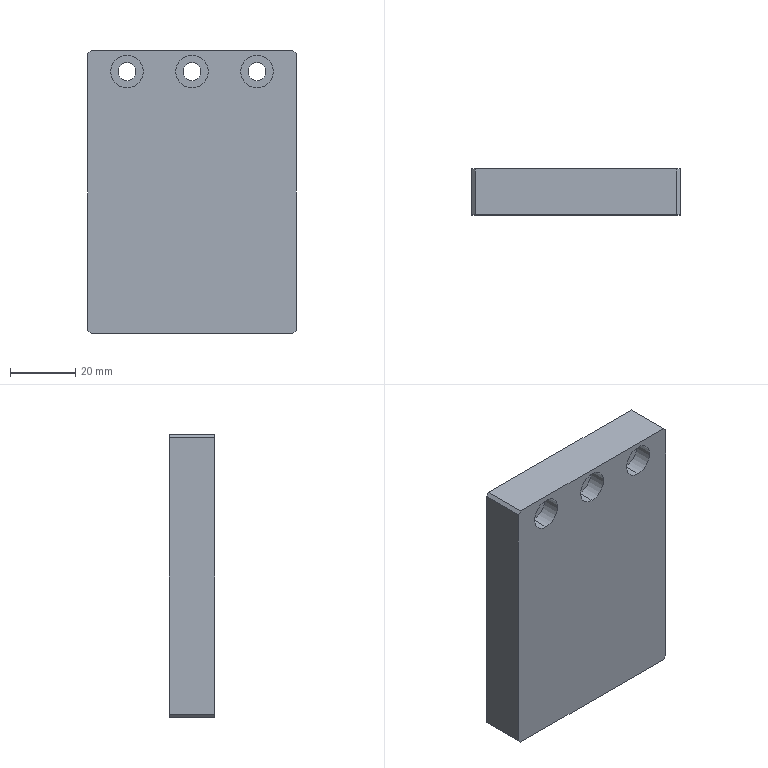Part | SolidWorks | features HoleWzd 2, Chamfer 1, Extrusion 1 | 1 solid | 37 faces | box 64 x 14 x 87 mm | volume 75198 mm3 | cylinder 18 | plane 13 | cone 6 | commonest cylinder face diameters 5 x6 5.5 x6 10 x6
STEP:
#1=CARTESIAN_POINT('',(32.5,-67.68,13.5));
#2=VERTEX_POINT('',#1);
#3=CARTESIAN_POINT('',(27.5,-67.68,13.5));
#4=VERTEX_POINT('',#3);
#5=CARTESIAN_POINT('',(30.,-67.68,13.5));
#6=DIRECTION('',(0.,0.,-1.));
#7=DIRECTION('',(-1.,0.,0.));
#8=AXIS2_PLACEMENT_3D('',#5,#6,#7);
#9=CIRCLE('',#8,2.5);
#10=EDGE_CURVE('',#2,#4,#9,.T.);
#11=ORIENTED_EDGE('',*,*,#10,.F.);
#12=CARTESIAN_POINT('',(32.5,-67.68,0.));
#13=VERTEX_POINT('',#12);
#14=CARTESIAN_POINT('',(32.5,-67.68,0.));
#15=DIRECTION('',(0.,0.,-1.));
#16=VECTOR('',#15,1000.);
#17=LINE('',#14,#16);
#18=EDGE_CURVE('',#2,#13,#17,.T.);
#19=ORIENTED_EDGE('',*,*,#18,.T.);
#20=CARTESIAN_POINT('',(27.5,-67.68,0.));
#21=VERTEX_POINT('',#20);
#22=CARTESIAN_POINT('',(30.,-67.68,0.));
#23=DIRECTION('',(0.,0.,-1.));
#24=DIRECTION('',(-1.,0.,0.));
#25=AXIS2_PLACEMENT_3D('',#22,#23,#24);
#26=CIRCLE('',#25,2.5);
#27=EDGE_CURVE('',#13,#21,#26,.T.);
#28=ORIENTED_EDGE('',*,*,#27,.T.);
#29=CARTESIAN_POINT('',(27.5,-67.68,0.));
#30=DIRECTION('',(0.,0.,-1.));
#31=VECTOR('',#30,1000.);
#32=LINE('',#29,#31);
#33=EDGE_CURVE('',#4,#21,#32,.T.);
#34=ORIENTED_EDGE('',*,*,#33,.F.);
#35=EDGE_LOOP('',(#11,#19,#28,#34));
#36=FACE_OUTER_BOUND('',#35,.T.);
#37=CARTESIAN_POINT('',(30.,-67.68,0.));
#38=DIRECTION('',(0.,0.,-1.));
#39=DIRECTION('',(-1.,0.,0.));
#40=AXIS2_PLACEMENT_3D('',#37,#38,#39);
#41=CYLINDRICAL_SURFACE('',#40,2.5);
#42=ADVANCED_FACE('',(#36),#41,.F.);
#43=CARTESIAN_POINT('',(30.,-67.68,15.002));
#44=VERTEX_POINT('',#43);
#45=CARTESIAN_POINT('',(27.5,-67.68,13.5));
#46=DIRECTION('',(-0.8572,0.,-0.515));
#47=VECTOR('',#46,1000.);
#48=LINE('',#45,#47);
#49=EDGE_CURVE('',#44,#4,#48,.T.);
#50=ORIENTED_EDGE('',*,*,#49,.F.);
#51=CARTESIAN_POINT('',(32.5,-67.68,13.5));
#52=DIRECTION('',(0.8572,0.,-0.515));
#53=VECTOR('',#52,1000.);
#54=LINE('',#51,#53);
#55=EDGE_CURVE('',#44,#2,#54,.T.);
#56=ORIENTED_EDGE('',*,*,#55,.T.);
#57=ORIENTED_EDGE('',*,*,#10,.T.);
#58=EDGE_LOOP('',(#50,#56,#57));
#59=FACE_OUTER_BOUND('',#58,.T.);
#60=CARTESIAN_POINT('',(30.,-67.68,13.5));
#61=DIRECTION('',(0.,0.,-1.));
#62=DIRECTION('',(-1.,0.,0.));
#63=AXIS2_PLACEMENT_3D('',#60,#61,#62);
#64=CONICAL_SURFACE('',#63,2.5,1.03);
#65=ADVANCED_FACE('',(#59),#64,.F.);
#66=CARTESIAN_POINT('',(12.5,-67.68,13.5));
#67=VERTEX_POINT('',#66);
#68=CARTESIAN_POINT('',(7.5,-67.68,13.5));
#69=VERTEX_POINT('',#68);
#70=CARTESIAN_POINT('',(10.,-67.68,13.5));
#71=DIRECTION('',(0.,0.,-1.));
#72=DIRECTION('',(-1.,0.,0.));
#73=AXIS2_PLACEMENT_3D('',#70,#71,#72);
#74=CIRCLE('',#73,2.5);
#75=EDGE_CURVE('',#67,#69,#74,.T.);
#76=ORIENTED_EDGE('',*,*,#75,.F.);
#77=CARTESIAN_POINT('',(12.5,-67.68,0.));
#78=VERTEX_POINT('',#77);
#79=CARTESIAN_POINT('',(12.5,-67.68,0.));
#80=DIRECTION('',(0.,0.,-1.));
#81=VECTOR('',#80,1000.);
#82=LINE('',#79,#81);
#83=EDGE_CURVE('',#67,#78,#82,.T.);
#84=ORIENTED_EDGE('',*,*,#83,.T.);
#85=CARTESIAN_POINT('',(7.5,-67.68,0.));
#86=VERTEX_POINT('',#85);
#87=CARTESIAN_POINT('',(10.,-67.68,0.));
#88=DIRECTION('',(0.,0.,-1.));
#89=DIRECTION('',(-1.,0.,0.));
#90=AXIS2_PLACEMENT_3D('',#87,#88,#89);
#91=CIRCLE('',#90,2.5);
#92=EDGE_CURVE('',#78,#86,#91,.T.);
#93=ORIENTED_EDGE('',*,*,#92,.T.);
#94=CARTESIAN_POINT('',(7.5,-67.68,0.));
#95=DIRECTION('',(0.,0.,-1.));
#96=VECTOR('',#95,1000.);
#97=LINE('',#94,#96);
#98=EDGE_CURVE('',#69,#86,#97,.T.);
#99=ORIENTED_EDGE('',*,*,#98,.F.);
#100=EDGE_LOOP('',(#76,#84,#93,#99));
#101=FACE_OUTER_BOUND('',#100,.T.);
#102=CARTESIAN_POINT('',(10.,-67.68,0.));
#103=DIRECTION('',(0.,0.,-1.));
#104=DIRECTION('',(-1.,0.,0.));
#105=AXIS2_PLACEMENT_3D('',#102,#103,#104);
#106=CYLINDRICAL_SURFACE('',#105,2.5);
#107=ADVANCED_FACE('',(#101),#106,.F.);
#108=CARTESIAN_POINT('',(10.,-67.68,15.002));
#109=VERTEX_POINT('',#108);
#110=CARTESIAN_POINT('',(7.5,-67.68,13.5));
#111=DIRECTION('',(-0.8572,0.,-0.515));
#112=VECTOR('',#111,1000.);
#113=LINE('',#110,#112);
#114=EDGE_CURVE('',#109,#69,#113,.T.);
#115=ORIENTED_EDGE('',*,*,#114,.F.);
#116=CARTESIAN_POINT('',(12.5,-67.68,13.5));
#117=DIRECTION('',(0.8572,0.,-0.515));
#118=VECTOR('',#117,1000.);
#119=LINE('',#116,#118);
#120=EDGE_CURVE('',#109,#67,#119,.T.);
#121=ORIENTED_EDGE('',*,*,#120,.T.);
#122=ORIENTED_EDGE('',*,*,#75,.T.);
#123=EDGE_LOOP('',(#115,#121,#122));
#124=FACE_OUTER_BOUND('',#123,.T.);
#125=CARTESIAN_POINT('',(10.,-67.68,13.5));
#126=DIRECTION('',(0.,0.,-1.));
#127=DIRECTION('',(-1.,0.,0.));
#128=AXIS2_PLACEMENT_3D('',#125,#126,#127);
#129=CONICAL_SURFACE('',#128,2.5,1.03);
#130=ADVANCED_FACE('',(#124),#129,.F.);
#131=CARTESIAN_POINT('',(-7.5,-67.68,13.5));
#132=VERTEX_POINT('',#131);
#133=CARTESIAN_POINT('',(-12.5,-67.68,13.5));
#134=VERTEX_POINT('',#133);
#135=CARTESIAN_POINT('',(-10.,-67.68,13.5));
#136=DIRECTION('',(0.,0.,-1.));
#137=DIRECTION('',(-1.,0.,0.));
#138=AXIS2_PLACEMENT_3D('',#135,#136,#137);
#139=CIRCLE('',#138,2.5);
#140=EDGE_CURVE('',#132,#134,#139,.T.);
#141=ORIENTED_EDGE('',*,*,#140,.F.);
#142=CARTESIAN_POINT('',(-7.5,-67.68,0.));
#143=VERTEX_POINT('',#142);
#144=CARTESIAN_POINT('',(-7.5,-67.68,0.));
#145=DIRECTION('',(0.,0.,-1.));
#146=VECTOR('',#145,1000.);
#147=LINE('',#144,#146);
#148=EDGE_CURVE('',#132,#143,#147,.T.);
#149=ORIENTED_EDGE('',*,*,#148,.T.);
#150=CARTESIAN_POINT('',(-12.5,-67.68,0.));
#151=VERTEX_POINT('',#150);
#152=CARTESIAN_POINT('',(-10.,-67.68,0.));
#153=DIRECTION('',(0.,0.,-1.));
#154=DIRECTION('',(-1.,0.,0.));
#155=AXIS2_PLACEMENT_3D('',#152,#153,#154);
#156=CIRCLE('',#155,2.5);
#157=EDGE_CURVE('',#143,#151,#156,.T.);
#158=ORIENTED_EDGE('',*,*,#157,.T.);
#159=CARTESIAN_POINT('',(-12.5,-67.68,0.));
#160=DIRECTION('',(0.,0.,-1.));
#161=VECTOR('',#160,1000.);
#162=LINE('',#159,#161);
#163=EDGE_CURVE('',#134,#151,#162,.T.);
#164=ORIENTED_EDGE('',*,*,#163,.F.);
#165=EDGE_LOOP('',(#141,#149,#158,#164));
#166=FACE_OUTER_BOUND('',#165,.T.);
#167=CARTESIAN_POINT('',(-10.,-67.68,0.));
#168=DIRECTION('',(0.,0.,-1.));
#169=DIRECTION('',(-1.,0.,0.));
#170=AXIS2_PLACEMENT_3D('',#167,#168,#169);
#171=CYLINDRICAL_SURFACE('',#170,2.5);
#172=ADVANCED_FACE('',(#166),#171,.F.);
#173=CARTESIAN_POINT('',(-10.,-67.68,15.002));
#174=VERTEX_POINT('',#173);
#175=CARTESIAN_POINT('',(-12.5,-67.68,13.5));
#176=DIRECTION('',(-0.8572,0.,-0.515));
#177=VECTOR('',#176,1000.);
#178=LINE('',#175,#177);
#179=EDGE_CURVE('',#174,#134,#178,.T.);
#180=ORIENTED_EDGE('',*,*,#179,.F.);
#181=CARTESIAN_POINT('',(-7.5,-67.68,13.5));
#182=DIRECTION('',(0.8572,0.,-0.515));
#183=VECTOR('',#182,1000.);
#184=LINE('',#181,#183);
#185=EDGE_CURVE('',#174,#132,#184,.T.);
#186=ORIENTED_EDGE('',*,*,#185,.T.);
#187=ORIENTED_EDGE('',*,*,#140,.T.);
#188=EDGE_LOOP('',(#180,#186,#187));
#189=FACE_OUTER_BOUND('',#188,.T.);
#190=CARTESIAN_POINT('',(-10.,-67.68,13.5));
#191=DIRECTION('',(0.,0.,-1.));
#192=DIRECTION('',(-1.,0.,0.));
#193=AXIS2_PLACEMENT_3D('',#190,#191,#192);
#194=CONICAL_SURFACE('',#193,2.5,1.03);
#195=ADVANCED_FACE('',(#189),#194,.F.);
#196=CARTESIAN_POINT('',(-10.,-69.18,85.5));
#197=VERTEX_POINT('',#196);
#198=CARTESIAN_POINT('',(-10.,-69.18,75.5));
#199=VERTEX_POINT('',#198);
#200=CARTESIAN_POINT('',(-10.,-69.18,80.5));
#201=DIRECTION('',(0.,-1.,0.));
#202=DIRECTION('',(0.,0.,-1.));
#203=AXIS2_PLACEMENT_3D('',#200,#201,#202);
#204=CIRCLE('',#203,5.);
#205=EDGE_CURVE('',#197,#199,#204,.T.);
#206=ORIENTED_EDGE('',*,*,#205,.F.);
#207=CARTESIAN_POINT('',(-10.,-74.68,85.5));
#208=VERTEX_POINT('',#207);
#209=CARTESIAN_POINT('',(-10.,-74.68,85.5));
#210=DIRECTION('',(0.,-1.,0.));
#211=VECTOR('',#210,1000.);
#212=LINE('',#209,#211);
#213=EDGE_CURVE('',#197,#208,#212,.T.);
#214=ORIENTED_EDGE('',*,*,#213,.T.);
#215=CARTESIAN_POINT('',(-10.,-74.68,75.5));
#216=VERTEX_POINT('',#215);
#217=CARTESIAN_POINT('',(-10.,-74.68,80.5));
#218=DIRECTION('',(0.,-1.,0.));
#219=DIRECTION('',(0.,0.,-1.));
#220=AXIS2_PLACEMENT_3D('',#217,#218,#219);
#221=CIRCLE('',#220,5.);
#222=EDGE_CURVE('',#208,#216,#221,.T.);
#223=ORIENTED_EDGE('',*,*,#222,.T.);
#224=CARTESIAN_POINT('',(-10.,-74.68,75.5));
#225=DIRECTION('',(0.,-1.,0.));
#226=VECTOR('',#225,1000.);
#227=LINE('',#224,#226);
#228=EDGE_CURVE('',#199,#216,#227,.T.);
#229=ORIENTED_EDGE('',*,*,#228,.F.);
#230=EDGE_LOOP('',(#206,#214,#223,#229));
#231=FACE_OUTER_BOUND('',#230,.T.);
#232=CARTESIAN_POINT('',(-10.,-74.68,80.5));
#233=DIRECTION('',(0.,-1.,0.));
#234=DIRECTION('',(0.,0.,-1.));
#235=AXIS2_PLACEMENT_3D('',#232,#233,#234);
#236=CYLINDRICAL_SURFACE('',#235,5.);
#237=ADVANCED_FACE('',(#231),#236,.F.);
#238=CARTESIAN_POINT('',(-10.,-60.68,83.25));
#239=VERTEX_POINT('',#238);
#240=CARTESIAN_POINT('',(-10.,-60.68,77.75));
#241=VERTEX_POINT('',#240);
#242=CARTESIAN_POINT('',(-10.,-60.68,80.5));
#243=DIRECTION('',(0.,-1.,0.));
#244=DIRECTION('',(0.,0.,-1.));
#245=AXIS2_PLACEMENT_3D('',#242,#243,#244);
#246=CIRCLE('',#245,2.75);
#247=EDGE_CURVE('',#239,#241,#246,.T.);
#248=ORIENTED_EDGE('',*,*,#247,.F.);
#249=CARTESIAN_POINT('',(-10.,-69.18,83.25));
#250=VERTEX_POINT('',#249);
#251=CARTESIAN_POINT('',(-10.,-74.68,83.25));
#252=DIRECTION('',(0.,-1.,0.));
#253=VECTOR('',#252,1000.);
#254=LINE('',#251,#253);
#255=EDGE_CURVE('',#239,#250,#254,.T.);
#256=ORIENTED_EDGE('',*,*,#255,.T.);
#257=CARTESIAN_POINT('',(-10.,-69.18,77.75));
#258=VERTEX_POINT('',#257);
#259=CARTESIAN_POINT('',(-10.,-69.18,80.5));
#260=DIRECTION('',(0.,-1.,0.));
#261=DIRECTION('',(0.,0.,-1.));
#262=AXIS2_PLACEMENT_3D('',#259,#260,#261);
#263=CIRCLE('',#262,2.75);
#264=EDGE_CURVE('',#250,#258,#263,.T.);
#265=ORIENTED_EDGE('',*,*,#264,.T.);
#266=CARTESIAN_POINT('',(-10.,-74.68,77.75));
#267=DIRECTION('',(0.,-1.,0.));
#268=VECTOR('',#267,1000.);
#269=LINE('',#266,#268);
#270=EDGE_CURVE('',#241,#258,#269,.T.);
#271=ORIENTED_EDGE('',*,*,#270,.F.);
#272=EDGE_LOOP('',(#248,#256,#265,#271));
#273=FACE_OUTER_BOUND('',#272,.T.);
#274=CARTESIAN_POINT('',(-10.,-74.68,80.5));
#275=DIRECTION('',(0.,-1.,0.));
#276=DIRECTION('',(0.,0.,-1.));
#277=AXIS2_PLACEMENT_3D('',#274,#275,#276);
#278=CYLINDRICAL_SURFACE('',#277,2.75);
#279=ADVANCED_FACE('',(#273),#278,.F.);
#280=CARTESIAN_POINT('',(10.,-69.18,85.5));
#281=VERTEX_POINT('',#280);
#282=CARTESIAN_POINT('',(10.,-69.18,75.5));
#283=VERTEX_POINT('',#282);
#284=CARTESIAN_POINT('',(10.,-69.18,80.5));
#285=DIRECTION('',(0.,-1.,0.));
#286=DIRECTION('',(0.,0.,-1.));
#287=AXIS2_PLACEMENT_3D('',#284,#285,#286);
#288=CIRCLE('',#287,5.);
#289=EDGE_CURVE('',#281,#283,#288,.T.);
#290=ORIENTED_EDGE('',*,*,#289,.F.);
#291=CARTESIAN_POINT('',(10.,-74.68,85.5));
#292=VERTEX_POINT('',#291);
#293=CARTESIAN_POINT('',(10.,-74.68,85.5));
#294=DIRECTION('',(0.,-1.,0.));
#295=VECTOR('',#294,1000.);
#296=LINE('',#293,#295);
#297=EDGE_CURVE('',#281,#292,#296,.T.);
#298=ORIENTED_EDGE('',*,*,#297,.T.);
#299=CARTESIAN_POINT('',(10.,-74.68,75.5));
#300=VERTEX_POINT('',#299);
#301=CARTESIAN_POINT('',(10.,-74.68,80.5));
#302=DIRECTION('',(0.,-1.,0.));
#303=DIRECTION('',(0.,0.,-1.));
#304=AXIS2_PLACEMENT_3D('',#301,#302,#303);
#305=CIRCLE('',#304,5.);
#306=EDGE_CURVE('',#292,#300,#305,.T.);
#307=ORIENTED_EDGE('',*,*,#306,.T.);
#308=CARTESIAN_POINT('',(10.,-74.68,75.5));
#309=DIRECTION('',(0.,-1.,0.));
#310=VECTOR('',#309,1000.);
#311=LINE('',#308,#310);
#312=EDGE_CURVE('',#283,#300,#311,.T.);
#313=ORIENTED_EDGE('',*,*,#312,.F.);
#314=EDGE_LOOP('',(#290,#298,#307,#313));
#315=FACE_OUTER_BOUND('',#314,.T.);
#316=CARTESIAN_POINT('',(10.,-74.68,80.5));
#317=DIRECTION('',(0.,-1.,0.));
#318=DIRECTION('',(0.,0.,-1.));
#319=AXIS2_PLACEMENT_3D('',#316,#317,#318);
#320=CYLINDRICAL_SURFACE('',#319,5.);
#321=ADVANCED_FACE('',(#315),#320,.F.);
#322=CARTESIAN_POINT('',(10.,-60.68,83.25));
#323=VERTEX_POINT('',#322);
#324=CARTESIAN_POINT('',(10.,-60.68,77.75));
#325=VERTEX_POINT('',#324);
#326=CARTESIAN_POINT('',(10.,-60.68,80.5));
#327=DIRECTION('',(0.,-1.,0.));
#328=DIRECTION('',(0.,0.,-1.));
#329=AXIS2_PLACEMENT_3D('',#326,#327,#328);
#330=CIRCLE('',#329,2.75);
#331=EDGE_CURVE('',#323,#325,#330,.T.);
#332=ORIENTED_EDGE('',*,*,#331,.F.);
#333=CARTESIAN_POINT('',(10.,-69.18,83.25));
#334=VERTEX_POINT('',#333);
#335=CARTESIAN_POINT('',(10.,-74.68,83.25));
#336=DIRECTION('',(0.,-1.,0.));
#337=VECTOR('',#336,1000.);
#338=LINE('',#335,#337);
#339=EDGE_CURVE('',#323,#334,#338,.T.);
#340=ORIENTED_EDGE('',*,*,#339,.T.);
#341=CARTESIAN_POINT('',(10.,-69.18,77.75));
#342=VERTEX_POINT('',#341);
#343=CARTESIAN_POINT('',(10.,-69.18,80.5));
#344=DIRECTION('',(0.,-1.,0.));
#345=DIRECTION('',(0.,0.,-1.));
#346=AXIS2_PLACEMENT_3D('',#343,#344,#345);
#347=CIRCLE('',#346,2.75);
#348=EDGE_CURVE('',#334,#342,#347,.T.);
#349=ORIENTED_EDGE('',*,*,#348,.T.);
#350=CARTESIAN_POINT('',(10.,-74.68,77.75));
#351=DIRECTION('',(0.,-1.,0.));
#352=VECTOR('',#351,1000.);
#353=LINE('',#350,#352);
#354=EDGE_CURVE('',#325,#342,#353,.T.);
#355=ORIENTED_EDGE('',*,*,#354,.F.);
#356=EDGE_LOOP('',(#332,#340,#349,#355));
#357=FACE_OUTER_BOUND('',#356,.T.);
#358=CARTESIAN_POINT('',(10.,-74.68,80.5));
#359=DIRECTION('',(0.,-1.,0.));
#360=DIRECTION('',(0.,0.,-1.));
#361=AXIS2_PLACEMENT_3D('',#358,#359,#360);
#362=CYLINDRICAL_SURFACE('',#361,2.75);
#363=ADVANCED_FACE('',(#357),#362,.F.);
#364=CARTESIAN_POINT('',(30.,-69.18,85.5));
#365=VERTEX_POINT('',#364);
#366=CARTESIAN_POINT('',(30.,-69.18,75.5));
#367=VERTEX_POINT('',#366);
#368=CARTESIAN_POINT('',(30.,-69.18,80.5));
#369=DIRECTION('',(0.,-1.,0.));
#370=DIRECTION('',(0.,0.,-1.));
#371=AXIS2_PLACEMENT_3D('',#368,#369,#370);
#372=CIRCLE('',#371,5.);
#373=EDGE_CURVE('',#365,#367,#372,.T.);
#374=ORIENTED_EDGE('',*,*,#373,.F.);
#375=CARTESIAN_POINT('',(30.,-74.68,85.5));
#376=VERTEX_POINT('',#375);
#377=CARTESIAN_POINT('',(30.,-74.68,85.5));
#378=DIRECTION('',(0.,-1.,0.));
#379=VECTOR('',#378,1000.);
#380=LINE('',#377,#379);
#381=EDGE_CURVE('',#365,#376,#380,.T.);
#382=ORIENTED_EDGE('',*,*,#381,.T.);
#383=CARTESIAN_POINT('',(30.,-74.68,75.5));
#384=VERTEX_POINT('',#383);
#385=CARTESIAN_POINT('',(30.,-74.68,80.5));
#386=DIRECTION('',(0.,-1.,0.));
#387=DIRECTION('',(0.,0.,-1.));
#388=AXIS2_PLACEMENT_3D('',#385,#386,#387);
#389=CIRCLE('',#388,5.);
#390=EDGE_CURVE('',#376,#384,#389,.T.);
#391=ORIENTED_EDGE('',*,*,#390,.T.);
#392=CARTESIAN_POINT('',(30.,-74.68,75.5));
#393=DIRECTION('',(0.,-1.,0.));
#394=VECTOR('',#393,1000.);
#395=LINE('',#392,#394);
#396=EDGE_CURVE('',#367,#384,#395,.T.);
#397=ORIENTED_EDGE('',*,*,#396,.F.);
#398=EDGE_LOOP('',(#374,#382,#391,#397));
#399=FACE_OUTER_BOUND('',#398,.T.);
#400=CARTESIAN_POINT('',(30.,-74.68,80.5));
#401=DIRECTION('',(0.,-1.,0.));
#402=DIRECTION('',(0.,0.,-1.));
#403=AXIS2_PLACEMENT_3D('',#400,#401,#402);
#404=CYLINDRICAL_SURFACE('',#403,5.);
#405=ADVANCED_FACE('',(#399),#404,.F.);
#406=CARTESIAN_POINT('',(30.,-60.68,83.25));
#407=VERTEX_POINT('',#406);
#408=CARTESIAN_POINT('',(30.,-60.68,77.75));
#409=VERTEX_POINT('',#408);
#410=CARTESIAN_POINT('',(30.,-60.68,80.5));
#411=DIRECTION('',(0.,-1.,0.));
#412=DIRECTION('',(0.,0.,-1.));
#413=AXIS2_PLACEMENT_3D('',#410,#411,#412);
#414=CIRCLE('',#413,2.75);
#415=EDGE_CURVE('',#407,#409,#414,.T.);
#416=ORIENTED_EDGE('',*,*,#415,.F.);
#417=CARTESIAN_POINT('',(30.,-69.18,83.25));
#418=VERTEX_POINT('',#417);
#419=CARTESIAN_POINT('',(30.,-74.68,83.25));
#420=DIRECTION('',(0.,-1.,0.));
#421=VECTOR('',#420,1000.);
#422=LINE('',#419,#421);
#423=EDGE_CURVE('',#407,#418,#422,.T.);
#424=ORIENTED_EDGE('',*,*,#423,.T.);
#425=CARTESIAN_POINT('',(30.,-69.18,77.75));
#426=VERTEX_POINT('',#425);
#427=CARTESIAN_POINT('',(30.,-69.18,80.5));
#428=DIRECTION('',(0.,-1.,0.));
#429=DIRECTION('',(0.,0.,-1.));
#430=AXIS2_PLACEMENT_3D('',#427,#428,#429);
#431=CIRCLE('',#430,2.75);
#432=EDGE_CURVE('',#418,#426,#431,.T.);
#433=ORIENTED_EDGE('',*,*,#432,.T.);
#434=CARTESIAN_POINT('',(30.,-74.68,77.75));
#435=DIRECTION('',(0.,-1.,0.));
#436=VECTOR('',#435,1000.);
#437=LINE('',#434,#436);
#438=EDGE_CURVE('',#409,#426,#437,.T.);
#439=ORIENTED_EDGE('',*,*,#438,.F.);
#440=EDGE_LOOP('',(#416,#424,#433,#439));
#441=FACE_OUTER_BOUND('',#440,.T.);
#442=CARTESIAN_POINT('',(30.,-74.68,80.5));
#443=DIRECTION('',(0.,-1.,0.));
#444=DIRECTION('',(0.,0.,-1.));
#445=AXIS2_PLACEMENT_3D('',#442,#443,#444);
#446=CYLINDRICAL_SURFACE('',#445,2.75);
#447=ADVANCED_FACE('',(#441),#446,.F.);
#448=CARTESIAN_POINT('',(-22.,-74.68,86.));
#449=VERTEX_POINT('',#448);
#450=CARTESIAN_POINT('',(-22.,-74.68,1.));
#451=VERTEX_POINT('',#450);
#452=CARTESIAN_POINT('',(-22.,-74.68,87.));
#453=DIRECTION('',(0.,0.,-1.));
#454=VECTOR('',#453,1000.);
#455=LINE('',#452,#454);
#456=EDGE_CURVE('',#449,#451,#455,.T.);
#457=ORIENTED_EDGE('',*,*,#456,.F.);
#458=CARTESIAN_POINT('',(-22.,-60.68,86.));
#459=VERTEX_POINT('',#458);
#460=CARTESIAN_POINT('',(-22.,-60.68,86.));
#461=DIRECTION('',(0.,1.,0.));
#462=VECTOR('',#461,1000.);
#463=LINE('',#460,#462);
#464=EDGE_CURVE('',#449,#459,#463,.T.);
#465=ORIENTED_EDGE('',*,*,#464,.T.);
#466=CARTESIAN_POINT('',(-22.,-60.68,1.));
#467=VERTEX_POINT('',#466);
#468=CARTESIAN_POINT('',(-22.,-60.68,87.));
#469=DIRECTION('',(0.,0.,-1.));
#470=VECTOR('',#469,1000.);
#471=LINE('',#468,#470);
#472=EDGE_CURVE('',#459,#467,#471,.T.);
#473=ORIENTED_EDGE('',*,*,#472,.T.);
#474=CARTESIAN_POINT('',(-22.,-60.68,1.));
#475=DIRECTION('',(0.,-1.,0.));
#476=VECTOR('',#475,1000.);
#477=LINE('',#474,#476);
#478=EDGE_CURVE('',#467,#451,#477,.T.);
#479=ORIENTED_EDGE('',*,*,#478,.T.);
#480=EDGE_LOOP('',(#457,#465,#473,#479));
#481=FACE_OUTER_BOUND('',#480,.T.);
#482=CARTESIAN_POINT('',(-22.,-60.68,87.));
#483=DIRECTION('',(1.,0.,0.));
#484=DIRECTION('',(0.,1.,0.));
#485=AXIS2_PLACEMENT_3D('',#482,#483,#484);
#486=PLANE('',#485);
#487=ADVANCED_FACE('',(#481),#486,.F.);
#488=CARTESIAN_POINT('',(-10.,-74.68,80.5));
#489=DIRECTION('',(0.,-1.,0.));
#490=DIRECTION('',(0.,0.,-1.));
#491=AXIS2_PLACEMENT_3D('',#488,#489,#490);
#492=CIRCLE('',#491,5.);
#493=EDGE_CURVE('',#216,#208,#492,.T.);
#494=ORIENTED_EDGE('',*,*,#493,.F.);
#495=ORIENTED_EDGE('',*,*,#222,.F.);
#496=EDGE_LOOP('',(#494,#495));
#497=FACE_BOUND('',#496,.T.);
#498=CARTESIAN_POINT('',(10.,-74.68,80.5));
#499=DIRECTION('',(0.,-1.,0.));
#500=DIRECTION('',(0.,0.,-1.));
#501=AXIS2_PLACEMENT_3D('',#498,#499,#500);
#502=CIRCLE('',#501,5.);
#503=EDGE_CURVE('',#300,#292,#502,.T.);
#504=ORIENTED_EDGE('',*,*,#503,.F.);
#505=ORIENTED_EDGE('',*,*,#306,.F.);
#506=EDGE_LOOP('',(#504,#505));
#507=FACE_BOUND('',#506,.T.);
#508=CARTESIAN_POINT('',(30.,-74.68,80.5));
#509=DIRECTION('',(0.,-1.,0.));
#510=DIRECTION('',(0.,0.,-1.));
#511=AXIS2_PLACEMENT_3D('',#508,#509,#510);
#512=CIRCLE('',#511,5.);
#513=EDGE_CURVE('',#384,#376,#512,.T.);
#514=ORIENTED_EDGE('',*,*,#513,.F.);
#515=ORIENTED_EDGE('',*,*,#390,.F.);
#516=EDGE_LOOP('',(#514,#515));
#517=FACE_BOUND('',#516,.T.);
#518=CARTESIAN_POINT('',(-21.,-74.68,87.));
#519=VERTEX_POINT('',#518);
#520=CARTESIAN_POINT('',(41.,-74.68,87.));
#521=VERTEX_POINT('',#520);
#522=CARTESIAN_POINT('',(-22.,-74.68,87.));
#523=DIRECTION('',(1.,0.,0.));
#524=VECTOR('',#523,1000.);
#525=LINE('',#522,#524);
#526=EDGE_CURVE('',#519,#521,#525,.T.);
#527=ORIENTED_EDGE('',*,*,#526,.F.);
#528=CARTESIAN_POINT('',(-21.,-74.68,87.));
#529=DIRECTION('',(-0.7071,0.,-0.7071));
#530=VECTOR('',#529,1000.);
#531=LINE('',#528,#530);
#532=EDGE_CURVE('',#519,#449,#531,.T.);
#533=ORIENTED_EDGE('',*,*,#532,.T.);
#534=ORIENTED_EDGE('',*,*,#456,.T.);
#535=CARTESIAN_POINT('',(-21.,-74.68,0.));
#536=VERTEX_POINT('',#535);
#537=CARTESIAN_POINT('',(-22.,-74.68,1.));
#538=DIRECTION('',(0.7071,0.,-0.7071));
#539=VECTOR('',#538,1000.);
#540=LINE('',#537,#539);
#541=EDGE_CURVE('',#451,#536,#540,.T.);
#542=ORIENTED_EDGE('',*,*,#541,.T.);
#543=CARTESIAN_POINT('',(41.,-74.68,0.));
#544=VERTEX_POINT('',#543);
#545=CARTESIAN_POINT('',(-22.,-74.68,0.));
#546=DIRECTION('',(1.,0.,0.));
#547=VECTOR('',#546,1000.);
#548=LINE('',#545,#547);
#549=EDGE_CURVE('',#536,#544,#548,.T.);
#550=ORIENTED_EDGE('',*,*,#549,.T.);
#551=CARTESIAN_POINT('',(42.,-74.68,1.));
#552=VERTEX_POINT('',#551);
#553=CARTESIAN_POINT('',(42.,-74.68,1.));
#554=DIRECTION('',(0.7071,0.,0.7071));
#555=VECTOR('',#554,1000.);
#556=LINE('',#553,#555);
#557=EDGE_CURVE('',#544,#552,#556,.T.);
#558=ORIENTED_EDGE('',*,*,#557,.T.);
#559=CARTESIAN_POINT('',(42.,-74.68,86.));
#560=VERTEX_POINT('',#559);
#561=CARTESIAN_POINT('',(42.,-74.68,87.));
#562=DIRECTION('',(0.,0.,-1.));
#563=VECTOR('',#562,1000.);
#564=LINE('',#561,#563);
#565=EDGE_CURVE('',#560,#552,#564,.T.);
#566=ORIENTED_EDGE('',*,*,#565,.F.);
#567=CARTESIAN_POINT('',(41.,-74.68,87.));
#568=DIRECTION('',(-0.7071,0.,0.7071));
#569=VECTOR('',#568,1000.);
#570=LINE('',#567,#569);
#571=EDGE_CURVE('',#560,#521,#570,.T.);
#572=ORIENTED_EDGE('',*,*,#571,.T.);
#573=EDGE_LOOP('',(#527,#533,#534,#542,#550,#558,#566,#572));
#574=FACE_OUTER_BOUND('',#573,.T.);
#575=CARTESIAN_POINT('',(-22.,-74.68,87.));
#576=DIRECTION('',(0.,1.,0.));
#577=DIRECTION('',(0.,0.,1.));
#578=AXIS2_PLACEMENT_3D('',#575,#576,#577);
#579=PLANE('',#578);
#580=ADVANCED_FACE('',(#497,#507,#517,#574),#579,.F.);
#581=CARTESIAN_POINT('',(42.,-60.68,86.));
#582=VERTEX_POINT('',#581);
#583=CARTESIAN_POINT('',(42.,-60.68,1.));
#584=VERTEX_POINT('',#583);
#585=CARTESIAN_POINT('',(42.,-60.68,87.));
#586=DIRECTION('',(0.,0.,-1.));
#587=VECTOR('',#586,1000.);
#588=LINE('',#585,#587);
#589=EDGE_CURVE('',#582,#584,#588,.T.);
#590=ORIENTED_EDGE('',*,*,#589,.F.);
#591=CARTESIAN_POINT('',(42.,-74.68,86.));
#592=DIRECTION('',(0.,-1.,0.));
#593=VECTOR('',#592,1000.);
#594=LINE('',#591,#593);
#595=EDGE_CURVE('',#582,#560,#594,.T.);
#596=ORIENTED_EDGE('',*,*,#595,.T.);
#597=ORIENTED_EDGE('',*,*,#565,.T.);
#598=CARTESIAN_POINT('',(42.,-60.68,1.));
#599=DIRECTION('',(0.,1.,0.));
#600=VECTOR('',#599,1000.);
#601=LINE('',#598,#600);
#602=EDGE_CURVE('',#552,#584,#601,.T.);
#603=ORIENTED_EDGE('',*,*,#602,.T.);
#604=EDGE_LOOP('',(#590,#596,#597,#603));
#605=FACE_OUTER_BOUND('',#604,.T.);
#606=CARTESIAN_POINT('',(42.,-60.68,87.));
#607=DIRECTION('',(-1.,0.,0.));
#608=DIRECTION('',(0.,0.,1.));
#609=AXIS2_PLACEMENT_3D('',#606,#607,#608);
#610=PLANE('',#609);
#611=ADVANCED_FACE('',(#605),#610,.F.);
#612=CARTESIAN_POINT('',(-10.,-60.68,80.5));
#613=DIRECTION('',(0.,-1.,0.));
#614=DIRECTION('',(0.,0.,-1.));
#615=AXIS2_PLACEMENT_3D('',#612,#613,#614);
#616=CIRCLE('',#615,2.75);
#617=EDGE_CURVE('',#241,#239,#616,.T.);
#618=ORIENTED_EDGE('',*,*,#617,.T.);
#619=ORIENTED_EDGE('',*,*,#247,.T.);
#620=EDGE_LOOP('',(#618,#619));
#621=FACE_BOUND('',#620,.T.);
#622=CARTESIAN_POINT('',(10.,-60.68,80.5));
#623=DIRECTION('',(0.,-1.,0.));
#624=DIRECTION('',(0.,0.,-1.));
#625=AXIS2_PLACEMENT_3D('',#622,#623,#624);
#626=CIRCLE('',#625,2.75);
#627=EDGE_CURVE('',#325,#323,#626,.T.);
#628=ORIENTED_EDGE('',*,*,#627,.T.);
#629=ORIENTED_EDGE('',*,*,#331,.T.);
#630=EDGE_LOOP('',(#628,#629));
#631=FACE_BOUND('',#630,.T.);
#632=CARTESIAN_POINT('',(30.,-60.68,80.5));
#633=DIRECTION('',(0.,-1.,0.));
#634=DIRECTION('',(0.,0.,-1.));
#635=AXIS2_PLACEMENT_3D('',#632,#633,#634);
#636=CIRCLE('',#635,2.75);
#637=EDGE_CURVE('',#409,#407,#636,.T.);
#638=ORIENTED_EDGE('',*,*,#637,.T.);
#639=ORIENTED_EDGE('',*,*,#415,.T.);
#640=EDGE_LOOP('',(#638,#639));
#641=FACE_BOUND('',#640,.T.);
#642=ORIENTED_EDGE('',*,*,#472,.F.);
#643=CARTESIAN_POINT('',(-21.,-60.68,87.));
#644=VERTEX_POINT('',#643);
#645=CARTESIAN_POINT('',(-21.,-60.68,87.));
#646=DIRECTION('',(0.7071,0.,0.7071));
#647=VECTOR('',#646,1000.);
#648=LINE('',#645,#647);
#649=EDGE_CURVE('',#459,#644,#648,.T.);
#650=ORIENTED_EDGE('',*,*,#649,.T.);
#651=CARTESIAN_POINT('',(41.,-60.68,87.));
#652=VERTEX_POINT('',#651);
#653=CARTESIAN_POINT('',(-22.,-60.68,87.));
#654=DIRECTION('',(-1.,0.,0.));
#655=VECTOR('',#654,1000.);
#656=LINE('',#653,#655);
#657=EDGE_CURVE('',#652,#644,#656,.T.);
#658=ORIENTED_EDGE('',*,*,#657,.F.);
#659=CARTESIAN_POINT('',(41.,-60.68,87.));
#660=DIRECTION('',(0.7071,0.,-0.7071));
#661=VECTOR('',#660,1000.);
#662=LINE('',#659,#661);
#663=EDGE_CURVE('',#652,#582,#662,.T.);
#664=ORIENTED_EDGE('',*,*,#663,.T.);
#665=ORIENTED_EDGE('',*,*,#589,.T.);
#666=CARTESIAN_POINT('',(41.,-60.68,0.));
#667=VERTEX_POINT('',#666);
#668=CARTESIAN_POINT('',(42.,-60.68,1.));
#669=DIRECTION('',(-0.7071,0.,-0.7071));
#670=VECTOR('',#669,1000.);
#671=LINE('',#668,#670);
#672=EDGE_CURVE('',#584,#667,#671,.T.);
#673=ORIENTED_EDGE('',*,*,#672,.T.);
#674=CARTESIAN_POINT('',(-21.,-60.68,0.));
#675=VERTEX_POINT('',#674);
#676=CARTESIAN_POINT('',(-22.,-60.68,0.));
#677=DIRECTION('',(-1.,0.,0.));
#678=VECTOR('',#677,1000.);
#679=LINE('',#676,#678);
#680=EDGE_CURVE('',#667,#675,#679,.T.);
#681=ORIENTED_EDGE('',*,*,#680,.T.);
#682=CARTESIAN_POINT('',(-22.,-60.68,1.));
#683=DIRECTION('',(-0.7071,0.,0.7071));
#684=VECTOR('',#683,1000.);
#685=LINE('',#682,#684);
#686=EDGE_CURVE('',#675,#467,#685,.T.);
#687=ORIENTED_EDGE('',*,*,#686,.T.);
#688=EDGE_LOOP('',(#642,#650,#658,#664,#665,#673,#681,#687));
#689=FACE_OUTER_BOUND('',#688,.T.);
#690=CARTESIAN_POINT('',(-22.,-60.68,87.));
#691=DIRECTION('',(0.,-1.,0.));
#692=DIRECTION('',(0.,0.,-1.));
#693=AXIS2_PLACEMENT_3D('',#690,#691,#692);
#694=PLANE('',#693);
#695=ADVANCED_FACE('',(#621,#631,#641,#689),#694,.F.);
#696=ORIENTED_EDGE('',*,*,#657,.T.);
#697=CARTESIAN_POINT('',(-21.,-74.68,87.));
#698=DIRECTION('',(0.,-1.,0.));
#699=VECTOR('',#698,1000.);
#700=LINE('',#697,#699);
#701=EDGE_CURVE('',#644,#519,#700,.T.);
#702=ORIENTED_EDGE('',*,*,#701,.T.);
#703=ORIENTED_EDGE('',*,*,#526,.T.);
#704=CARTESIAN_POINT('',(41.,-60.68,87.));
#705=DIRECTION('',(0.,1.,0.));
#706=VECTOR('',#705,1000.);
#707=LINE('',#704,#706);
#708=EDGE_CURVE('',#521,#652,#707,.T.);
#709=ORIENTED_EDGE('',*,*,#708,.T.);
#710=EDGE_LOOP('',(#696,#702,#703,#709));
#711=FACE_OUTER_BOUND('',#710,.T.);
#712=CARTESIAN_POINT('',(0.,0.,87.));
#713=DIRECTION('',(0.,0.,1.));
#714=DIRECTION('',(1.,0.,0.));
#715=AXIS2_PLACEMENT_3D('',#712,#713,#714);
#716=PLANE('',#715);
#717=ADVANCED_FACE('',(#711),#716,.T.);
#718=CARTESIAN_POINT('',(30.,-67.68,0.));
#719=DIRECTION('',(0.,0.,-1.));
#720=DIRECTION('',(-1.,0.,0.));
#721=AXIS2_PLACEMENT_3D('',#718,#719,#720);
#722=CIRCLE('',#721,2.5);
#723=EDGE_CURVE('',#21,#13,#722,.T.);
#724=ORIENTED_EDGE('',*,*,#723,.F.);
#725=ORIENTED_EDGE('',*,*,#27,.F.);
#726=EDGE_LOOP('',(#724,#725));
#727=FACE_BOUND('',#726,.T.);
#728=CARTESIAN_POINT('',(10.,-67.68,0.));
#729=DIRECTION('',(0.,0.,-1.));
#730=DIRECTION('',(-1.,0.,0.));
#731=AXIS2_PLACEMENT_3D('',#728,#729,#730);
#732=CIRCLE('',#731,2.5);
#733=EDGE_CURVE('',#86,#78,#732,.T.);
#734=ORIENTED_EDGE('',*,*,#733,.F.);
#735=ORIENTED_EDGE('',*,*,#92,.F.);
#736=EDGE_LOOP('',(#734,#735));
#737=FACE_BOUND('',#736,.T.);
#738=CARTESIAN_POINT('',(-10.,-67.68,0.));
#739=DIRECTION('',(0.,0.,-1.));
#740=DIRECTION('',(-1.,0.,0.));
#741=AXIS2_PLACEMENT_3D('',#738,#739,#740);
#742=CIRCLE('',#741,2.5);
#743=EDGE_CURVE('',#151,#143,#742,.T.);
#744=ORIENTED_EDGE('',*,*,#743,.F.);
#745=ORIENTED_EDGE('',*,*,#157,.F.);
#746=EDGE_LOOP('',(#744,#745));
#747=FACE_BOUND('',#746,.T.);
#748=ORIENTED_EDGE('',*,*,#549,.F.);
#749=CARTESIAN_POINT('',(-21.,0.,0.));
#750=DIRECTION('',(0.,1.,0.));
#751=VECTOR('',#750,1000.);
#752=LINE('',#749,#751);
#753=EDGE_CURVE('',#536,#675,#752,.T.);
#754=ORIENTED_EDGE('',*,*,#753,.T.);
#755=ORIENTED_EDGE('',*,*,#680,.F.);
#756=CARTESIAN_POINT('',(41.,0.,0.));
#757=DIRECTION('',(0.,-1.,0.));
#758=VECTOR('',#757,1000.);
#759=LINE('',#756,#758);
#760=EDGE_CURVE('',#667,#544,#759,.T.);
#761=ORIENTED_EDGE('',*,*,#760,.T.);
#762=EDGE_LOOP('',(#748,#754,#755,#761));
#763=FACE_OUTER_BOUND('',#762,.T.);
#764=CARTESIAN_POINT('',(0.,0.,0.));
#765=DIRECTION('',(0.,0.,1.));
#766=DIRECTION('',(1.,0.,0.));
#767=AXIS2_PLACEMENT_3D('',#764,#765,#766);
#768=PLANE('',#767);
#769=ADVANCED_FACE('',(#727,#737,#747,#763),#768,.F.);
#770=ORIENTED_EDGE('',*,*,#423,.F.);
#771=ORIENTED_EDGE('',*,*,#637,.F.);
#772=ORIENTED_EDGE('',*,*,#438,.T.);
#773=CARTESIAN_POINT('',(30.,-69.18,80.5));
#774=DIRECTION('',(0.,-1.,0.));
#775=DIRECTION('',(0.,0.,-1.));
#776=AXIS2_PLACEMENT_3D('',#773,#774,#775);
#777=CIRCLE('',#776,2.75);
#778=EDGE_CURVE('',#426,#418,#777,.T.);
#779=ORIENTED_EDGE('',*,*,#778,.T.);
#780=EDGE_LOOP('',(#770,#771,#772,#779));
#781=FACE_OUTER_BOUND('',#780,.T.);
#782=CARTESIAN_POINT('',(30.,-74.68,80.5));
#783=DIRECTION('',(0.,-1.,0.));
#784=DIRECTION('',(0.,0.,-1.));
#785=AXIS2_PLACEMENT_3D('',#782,#783,#784);
#786=CYLINDRICAL_SURFACE('',#785,2.75);
#787=ADVANCED_FACE('',(#781),#786,.F.);
#788=ORIENTED_EDGE('',*,*,#778,.F.);
#789=ORIENTED_EDGE('',*,*,#432,.F.);
#790=EDGE_LOOP('',(#788,#789));
#791=FACE_BOUND('',#790,.T.);
#792=CARTESIAN_POINT('',(30.,-69.18,80.5));
#793=DIRECTION('',(0.,-1.,0.));
#794=DIRECTION('',(0.,0.,-1.));
#795=AXIS2_PLACEMENT_3D('',#792,#793,#794);
#796=CIRCLE('',#795,5.);
#797=EDGE_CURVE('',#367,#365,#796,.T.);
#798=ORIENTED_EDGE('',*,*,#797,.T.);
#799=ORIENTED_EDGE('',*,*,#373,.T.);
#800=EDGE_LOOP('',(#798,#799));
#801=FACE_OUTER_BOUND('',#800,.T.);
#802=CARTESIAN_POINT('',(32.75,-69.18,80.5));
#803=DIRECTION('',(0.,1.,0.));
#804=DIRECTION('',(0.,0.,1.));
#805=AXIS2_PLACEMENT_3D('',#802,#803,#804);
#806=PLANE('',#805);
#807=ADVANCED_FACE('',(#791,#801),#806,.F.);
#808=ORIENTED_EDGE('',*,*,#381,.F.);
#809=ORIENTED_EDGE('',*,*,#797,.F.);
#810=ORIENTED_EDGE('',*,*,#396,.T.);
#811=ORIENTED_EDGE('',*,*,#513,.T.);
#812=EDGE_LOOP('',(#808,#809,#810,#811));
#813=FACE_OUTER_BOUND('',#812,.T.);
#814=CARTESIAN_POINT('',(30.,-74.68,80.5));
#815=DIRECTION('',(0.,-1.,0.));
#816=DIRECTION('',(0.,0.,-1.));
#817=AXIS2_PLACEMENT_3D('',#814,#815,#816);
#818=CYLINDRICAL_SURFACE('',#817,5.);
#819=ADVANCED_FACE('',(#813),#818,.F.);
#820=ORIENTED_EDGE('',*,*,#339,.F.);
#821=ORIENTED_EDGE('',*,*,#627,.F.);
#822=ORIENTED_EDGE('',*,*,#354,.T.);
#823=CARTESIAN_POINT('',(10.,-69.18,80.5));
#824=DIRECTION('',(0.,-1.,0.));
#825=DIRECTION('',(0.,0.,-1.));
#826=AXIS2_PLACEMENT_3D('',#823,#824,#825);
#827=CIRCLE('',#826,2.75);
#828=EDGE_CURVE('',#342,#334,#827,.T.);
#829=ORIENTED_EDGE('',*,*,#828,.T.);
#830=EDGE_LOOP('',(#820,#821,#822,#829));
#831=FACE_OUTER_BOUND('',#830,.T.);
#832=CARTESIAN_POINT('',(10.,-74.68,80.5));
#833=DIRECTION('',(0.,-1.,0.));
#834=DIRECTION('',(0.,0.,-1.));
#835=AXIS2_PLACEMENT_3D('',#832,#833,#834);
#836=CYLINDRICAL_SURFACE('',#835,2.75);
#837=ADVANCED_FACE('',(#831),#836,.F.);
#838=ORIENTED_EDGE('',*,*,#828,.F.);
#839=ORIENTED_EDGE('',*,*,#348,.F.);
#840=EDGE_LOOP('',(#838,#839));
#841=FACE_BOUND('',#840,.T.);
#842=CARTESIAN_POINT('',(10.,-69.18,80.5));
#843=DIRECTION('',(0.,-1.,0.));
#844=DIRECTION('',(0.,0.,-1.));
#845=AXIS2_PLACEMENT_3D('',#842,#843,#844);
#846=CIRCLE('',#845,5.);
#847=EDGE_CURVE('',#283,#281,#846,.T.);
#848=ORIENTED_EDGE('',*,*,#847,.T.);
#849=ORIENTED_EDGE('',*,*,#289,.T.);
#850=EDGE_LOOP('',(#848,#849));
#851=FACE_OUTER_BOUND('',#850,.T.);
#852=CARTESIAN_POINT('',(12.75,-69.18,80.5));
#853=DIRECTION('',(0.,1.,0.));
#854=DIRECTION('',(0.,0.,1.));
#855=AXIS2_PLACEMENT_3D('',#852,#853,#854);
#856=PLANE('',#855);
#857=ADVANCED_FACE('',(#841,#851),#856,.F.);
#858=ORIENTED_EDGE('',*,*,#297,.F.);
#859=ORIENTED_EDGE('',*,*,#847,.F.);
#860=ORIENTED_EDGE('',*,*,#312,.T.);
#861=ORIENTED_EDGE('',*,*,#503,.T.);
#862=EDGE_LOOP('',(#858,#859,#860,#861));
#863=FACE_OUTER_BOUND('',#862,.T.);
#864=CARTESIAN_POINT('',(10.,-74.68,80.5));
#865=DIRECTION('',(0.,-1.,0.));
#866=DIRECTION('',(0.,0.,-1.));
#867=AXIS2_PLACEMENT_3D('',#864,#865,#866);
#868=CYLINDRICAL_SURFACE('',#867,5.);
#869=ADVANCED_FACE('',(#863),#868,.F.);
#870=ORIENTED_EDGE('',*,*,#255,.F.);
#871=ORIENTED_EDGE('',*,*,#617,.F.);
#872=ORIENTED_EDGE('',*,*,#270,.T.);
#873=CARTESIAN_POINT('',(-10.,-69.18,80.5));
#874=DIRECTION('',(0.,-1.,0.));
#875=DIRECTION('',(0.,0.,-1.));
#876=AXIS2_PLACEMENT_3D('',#873,#874,#875);
#877=CIRCLE('',#876,2.75);
#878=EDGE_CURVE('',#258,#250,#877,.T.);
#879=ORIENTED_EDGE('',*,*,#878,.T.);
#880=EDGE_LOOP('',(#870,#871,#872,#879));
#881=FACE_OUTER_BOUND('',#880,.T.);
#882=CARTESIAN_POINT('',(-10.,-74.68,80.5));
#883=DIRECTION('',(0.,-1.,0.));
#884=DIRECTION('',(0.,0.,-1.));
#885=AXIS2_PLACEMENT_3D('',#882,#883,#884);
#886=CYLINDRICAL_SURFACE('',#885,2.75);
#887=ADVANCED_FACE('',(#881),#886,.F.);
#888=ORIENTED_EDGE('',*,*,#878,.F.);
#889=ORIENTED_EDGE('',*,*,#264,.F.);
#890=EDGE_LOOP('',(#888,#889));
#891=FACE_BOUND('',#890,.T.);
#892=CARTESIAN_POINT('',(-10.,-69.18,80.5));
#893=DIRECTION('',(0.,-1.,0.));
#894=DIRECTION('',(0.,0.,-1.));
#895=AXIS2_PLACEMENT_3D('',#892,#893,#894);
#896=CIRCLE('',#895,5.);
#897=EDGE_CURVE('',#199,#197,#896,.T.);
#898=ORIENTED_EDGE('',*,*,#897,.T.);
#899=ORIENTED_EDGE('',*,*,#205,.T.);
#900=EDGE_LOOP('',(#898,#899));
#901=FACE_OUTER_BOUND('',#900,.T.);
#902=CARTESIAN_POINT('',(-7.25,-69.18,80.5));
#903=DIRECTION('',(0.,1.,0.));
#904=DIRECTION('',(0.,0.,1.));
#905=AXIS2_PLACEMENT_3D('',#902,#903,#904);
#906=PLANE('',#905);
#907=ADVANCED_FACE('',(#891,#901),#906,.F.);
#908=ORIENTED_EDGE('',*,*,#213,.F.);
#909=ORIENTED_EDGE('',*,*,#897,.F.);
#910=ORIENTED_EDGE('',*,*,#228,.T.);
#911=ORIENTED_EDGE('',*,*,#493,.T.);
#912=EDGE_LOOP('',(#908,#909,#910,#911));
#913=FACE_OUTER_BOUND('',#912,.T.);
#914=CARTESIAN_POINT('',(-10.,-74.68,80.5));
#915=DIRECTION('',(0.,-1.,0.));
#916=DIRECTION('',(0.,0.,-1.));
#917=AXIS2_PLACEMENT_3D('',#914,#915,#916);
#918=CYLINDRICAL_SURFACE('',#917,5.);
#919=ADVANCED_FACE('',(#913),#918,.F.);
#920=ORIENTED_EDGE('',*,*,#185,.F.);
#921=ORIENTED_EDGE('',*,*,#179,.T.);
#922=CARTESIAN_POINT('',(-10.,-67.68,13.5));
#923=DIRECTION('',(0.,0.,-1.));
#924=DIRECTION('',(-1.,0.,0.));
#925=AXIS2_PLACEMENT_3D('',#922,#923,#924);
#926=CIRCLE('',#925,2.5);
#927=EDGE_CURVE('',#134,#132,#926,.T.);
#928=ORIENTED_EDGE('',*,*,#927,.T.);
#929=EDGE_LOOP('',(#920,#921,#928));
#930=FACE_OUTER_BOUND('',#929,.T.);
#931=CARTESIAN_POINT('',(-10.,-67.68,13.5));
#932=DIRECTION('',(0.,0.,-1.));
#933=DIRECTION('',(-1.,0.,0.));
#934=AXIS2_PLACEMENT_3D('',#931,#932,#933);
#935=CONICAL_SURFACE('',#934,2.5,1.03);
#936=ADVANCED_FACE('',(#930),#935,.F.);
#937=ORIENTED_EDGE('',*,*,#148,.F.);
#938=ORIENTED_EDGE('',*,*,#927,.F.);
#939=ORIENTED_EDGE('',*,*,#163,.T.);
#940=ORIENTED_EDGE('',*,*,#743,.T.);
#941=EDGE_LOOP('',(#937,#938,#939,#940));
#942=FACE_OUTER_BOUND('',#941,.T.);
#943=CARTESIAN_POINT('',(-10.,-67.68,0.));
#944=DIRECTION('',(0.,0.,-1.));
#945=DIRECTION('',(-1.,0.,0.));
#946=AXIS2_PLACEMENT_3D('',#943,#944,#945);
#947=CYLINDRICAL_SURFACE('',#946,2.5);
#948=ADVANCED_FACE('',(#942),#947,.F.);
#949=ORIENTED_EDGE('',*,*,#120,.F.);
#950=ORIENTED_EDGE('',*,*,#114,.T.);
#951=CARTESIAN_POINT('',(10.,-67.68,13.5));
#952=DIRECTION('',(0.,0.,-1.));
#953=DIRECTION('',(-1.,0.,0.));
#954=AXIS2_PLACEMENT_3D('',#951,#952,#953);
#955=CIRCLE('',#954,2.5);
#956=EDGE_CURVE('',#69,#67,#955,.T.);
#957=ORIENTED_EDGE('',*,*,#956,.T.);
#958=EDGE_LOOP('',(#949,#950,#957));
#959=FACE_OUTER_BOUND('',#958,.T.);
#960=CARTESIAN_POINT('',(10.,-67.68,13.5));
#961=DIRECTION('',(0.,0.,-1.));
#962=DIRECTION('',(-1.,0.,0.));
#963=AXIS2_PLACEMENT_3D('',#960,#961,#962);
#964=CONICAL_SURFACE('',#963,2.5,1.03);
#965=ADVANCED_FACE('',(#959),#964,.F.);
#966=ORIENTED_EDGE('',*,*,#83,.F.);
#967=ORIENTED_EDGE('',*,*,#956,.F.);
#968=ORIENTED_EDGE('',*,*,#98,.T.);
#969=ORIENTED_EDGE('',*,*,#733,.T.);
#970=EDGE_LOOP('',(#966,#967,#968,#969));
#971=FACE_OUTER_BOUND('',#970,.T.);
#972=CARTESIAN_POINT('',(10.,-67.68,0.));
#973=DIRECTION('',(0.,0.,-1.));
#974=DIRECTION('',(-1.,0.,0.));
#975=AXIS2_PLACEMENT_3D('',#972,#973,#974);
#976=CYLINDRICAL_SURFACE('',#975,2.5);
#977=ADVANCED_FACE('',(#971),#976,.F.);
#978=ORIENTED_EDGE('',*,*,#55,.F.);
#979=ORIENTED_EDGE('',*,*,#49,.T.);
#980=CARTESIAN_POINT('',(30.,-67.68,13.5));
#981=DIRECTION('',(0.,0.,-1.));
#982=DIRECTION('',(-1.,0.,0.));
#983=AXIS2_PLACEMENT_3D('',#980,#981,#982);
#984=CIRCLE('',#983,2.5);
#985=EDGE_CURVE('',#4,#2,#984,.T.);
#986=ORIENTED_EDGE('',*,*,#985,.T.);
#987=EDGE_LOOP('',(#978,#979,#986));
#988=FACE_OUTER_BOUND('',#987,.T.);
#989=CARTESIAN_POINT('',(30.,-67.68,13.5));
#990=DIRECTION('',(0.,0.,-1.));
#991=DIRECTION('',(-1.,0.,0.));
#992=AXIS2_PLACEMENT_3D('',#989,#990,#991);
#993=CONICAL_SURFACE('',#992,2.5,1.03);
#994=ADVANCED_FACE('',(#988),#993,.F.);
#995=ORIENTED_EDGE('',*,*,#18,.F.);
#996=ORIENTED_EDGE('',*,*,#985,.F.);
#997=ORIENTED_EDGE('',*,*,#33,.T.);
#998=ORIENTED_EDGE('',*,*,#723,.T.);
#999=EDGE_LOOP('',(#995,#996,#997,#998));
#1000=FACE_OUTER_BOUND('',#999,.T.);
#1001=CARTESIAN_POINT('',(30.,-67.68,0.));
#1002=DIRECTION('',(0.,0.,-1.));
#1003=DIRECTION('',(-1.,0.,0.));
#1004=AXIS2_PLACEMENT_3D('',#1001,#1002,#1003);
#1005=CYLINDRICAL_SURFACE('',#1004,2.5);
#1006=ADVANCED_FACE('',(#1000),#1005,.F.);
#1007=ORIENTED_EDGE('',*,*,#649,.F.);
#1008=ORIENTED_EDGE('',*,*,#464,.F.);
#1009=ORIENTED_EDGE('',*,*,#532,.F.);
#1010=ORIENTED_EDGE('',*,*,#701,.F.);
#1011=EDGE_LOOP('',(#1007,#1008,#1009,#1010));
#1012=FACE_OUTER_BOUND('',#1011,.T.);
#1013=CARTESIAN_POINT('',(-21.,0.,87.));
#1014=DIRECTION('',(-0.7071,0.,0.7071));
#1015=DIRECTION('',(0.,1.,0.));
#1016=AXIS2_PLACEMENT_3D('',#1013,#1014,#1015);
#1017=PLANE('',#1016);
#1018=ADVANCED_FACE('',(#1012),#1017,.T.);
#1019=ORIENTED_EDGE('',*,*,#571,.F.);
#1020=ORIENTED_EDGE('',*,*,#595,.F.);
#1021=ORIENTED_EDGE('',*,*,#663,.F.);
#1022=ORIENTED_EDGE('',*,*,#708,.F.);
#1023=EDGE_LOOP('',(#1019,#1020,#1021,#1022));
#1024=FACE_OUTER_BOUND('',#1023,.T.);
#1025=CARTESIAN_POINT('',(41.,0.,87.));
#1026=DIRECTION('',(0.7071,0.,0.7071));
#1027=DIRECTION('',(0.,-1.,0.));
#1028=AXIS2_PLACEMENT_3D('',#1025,#1026,#1027);
#1029=PLANE('',#1028);
#1030=ADVANCED_FACE('',(#1024),#1029,.T.);
#1031=ORIENTED_EDGE('',*,*,#686,.F.);
#1032=ORIENTED_EDGE('',*,*,#753,.F.);
#1033=ORIENTED_EDGE('',*,*,#541,.F.);
#1034=ORIENTED_EDGE('',*,*,#478,.F.);
#1035=EDGE_LOOP('',(#1031,#1032,#1033,#1034));
#1036=FACE_OUTER_BOUND('',#1035,.T.);
#1037=CARTESIAN_POINT('',(-22.,-60.68,1.));
#1038=DIRECTION('',(0.7071,0.,0.7071));
#1039=DIRECTION('',(0.,-1.,0.));
#1040=AXIS2_PLACEMENT_3D('',#1037,#1038,#1039);
#1041=PLANE('',#1040);
#1042=ADVANCED_FACE('',(#1036),#1041,.F.);
#1043=ORIENTED_EDGE('',*,*,#557,.F.);
#1044=ORIENTED_EDGE('',*,*,#760,.F.);
#1045=ORIENTED_EDGE('',*,*,#672,.F.);
#1046=ORIENTED_EDGE('',*,*,#602,.F.);
#1047=EDGE_LOOP('',(#1043,#1044,#1045,#1046));
#1048=FACE_OUTER_BOUND('',#1047,.T.);
#1049=CARTESIAN_POINT('',(42.,-60.68,1.));
#1050=DIRECTION('',(-0.7071,0.,0.7071));
#1051=DIRECTION('',(0.,1.,0.));
#1052=AXIS2_PLACEMENT_3D('',#1049,#1050,#1051);
#1053=PLANE('',#1052);
#1054=ADVANCED_FACE('',(#1048),#1053,.F.);
#1055=CLOSED_SHELL('',(#42,#65,#107,#130,#172,#195,#237,#279,#321,#363,#405,#447,#487,#580,#611,#695,#717,#769,#787,#807,#819,#837,#857,#869,#887,#907,#919,#936,#948,#965,#977,#994,#1006,#1018,#1030,#1042,#1054));
#1056=MANIFOLD_SOLID_BREP('',#1055);
#1057=CARTESIAN_POINT('',(0.,0.,0.));
#1058=DIRECTION('',(0.,0.,1.));
#1059=DIRECTION('',(1.,0.,0.));
#1060=AXIS2_PLACEMENT_3D('',#1057,#1058,#1059);
#1061=(LENGTH_UNIT()NAMED_UNIT(*)SI_UNIT(.MILLI.,.METRE.));
#1062=UNCERTAINTY_MEASURE_WITH_UNIT(LENGTH_MEASURE(0.00001),#1061,'','');
#1063=(NAMED_UNIT(*)PLANE_ANGLE_UNIT()SI_UNIT($,.RADIAN.));
#1064=(NAMED_UNIT(*)SI_UNIT($,.STERADIAN.)SOLID_ANGLE_UNIT());
#1065=(GEOMETRIC_REPRESENTATION_CONTEXT(3)GLOBAL_UNCERTAINTY_ASSIGNED_CONTEXT((#1062))GLOBAL_UNIT_ASSIGNED_CONTEXT((#1061,#1063,#1064))REPRESENTATION_CONTEXT('',''));
#1066=ADVANCED_BREP_SHAPE_REPRESENTATION('',(#1056,#1060),#1065);